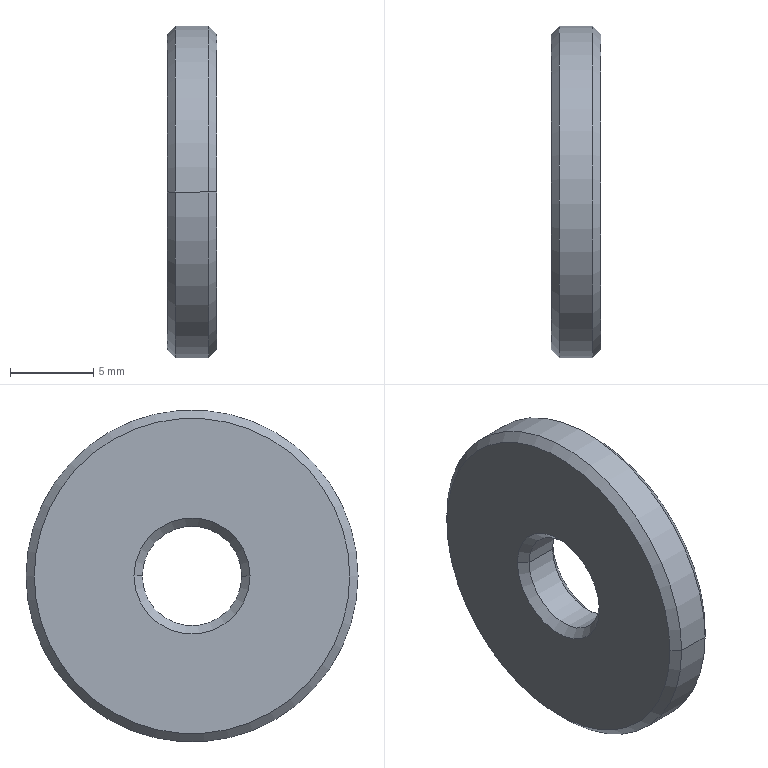Part | STEP file | 0245_005_WSSB20-6-3 | 1 solid | 14 faces | box 3 x 20 x 20 mm | volume 837.234 mm3 | cone 8 | cylinder 4 | plane 2 | commonest cylinder face diameters 6 x2 20 x2
STEP:
#1=CARTESIAN_POINT('',(0.,0.,0.));
#2=DIRECTION('',(0.,0.,1.));
#3=DIRECTION('',(1.,0.,0.));
#4=AXIS2_PLACEMENT_3D('',#1,#2,#3);
#5=CARTESIAN_POINT('',(0.5,-3.,0.));
#6=VERTEX_POINT('',#5);
#7=CARTESIAN_POINT('',(0.,-3.5,0.));
#8=VERTEX_POINT('',#7);
#9=CARTESIAN_POINT('',(0.,-3.5,0.));
#10=DIRECTION('',(-0.7071,-0.7071,0.));
#11=VECTOR('',#10,1.);
#12=LINE('',#9,#11);
#13=CARTESIAN_POINT('',(0.,0.,0.));
#14=DIRECTION('',(-1.,0.,0.));
#15=DIRECTION('',(0.,-1.,0.));
#16=AXIS2_PLACEMENT_3D('',#13,#14,#15);
#17=CONICAL_SURFACE('',#16,3.5,0.7854);
#18=CARTESIAN_POINT('',(6.283,0.));
#19=DIRECTION('',(0.,1.));
#20=VECTOR('',#19,1.);
#21=LINE('',#18,#20);
#22=(GEOMETRIC_REPRESENTATION_CONTEXT(2)PARAMETRIC_REPRESENTATION_CONTEXT()REPRESENTATION_CONTEXT('',''));
#23=DEFINITIONAL_REPRESENTATION('',(#21),#22);
#24=PCURVE('',#17,#23);
#25=CARTESIAN_POINT('',(0.,0.,0.));
#26=DIRECTION('',(-1.,0.,0.));
#27=DIRECTION('',(0.,-1.,0.));
#28=AXIS2_PLACEMENT_3D('',#25,#26,#27);
#29=CONICAL_SURFACE('',#28,3.5,0.7854);
#30=CARTESIAN_POINT('',(0.,0.));
#31=DIRECTION('',(0.,1.));
#32=VECTOR('',#31,1.);
#33=LINE('',#30,#32);
#34=(GEOMETRIC_REPRESENTATION_CONTEXT(2)PARAMETRIC_REPRESENTATION_CONTEXT()REPRESENTATION_CONTEXT('',''));
#35=DEFINITIONAL_REPRESENTATION('',(#33),#34);
#36=PCURVE('',#29,#35);
#37=SURFACE_CURVE('',#12,(#24,#36),.PCURVE_S1.);
#38=EDGE_CURVE('',#6,#8,#37,.T.);
#39=ORIENTED_EDGE('',*,*,#38,.T.);
#40=CARTESIAN_POINT('',(0.,3.5,0.));
#41=VERTEX_POINT('',#40);
#42=CARTESIAN_POINT('',(0.,0.,0.));
#43=DIRECTION('',(1.,0.,0.));
#44=DIRECTION('',(0.,-1.,0.));
#45=AXIS2_PLACEMENT_3D('',#42,#43,#44);
#46=CIRCLE('',#45,3.5);
#47=CARTESIAN_POINT('',(6.283,0.));
#48=DIRECTION('',(-1.,0.));
#49=VECTOR('',#48,1.);
#50=LINE('',#47,#49);
#51=(GEOMETRIC_REPRESENTATION_CONTEXT(2)PARAMETRIC_REPRESENTATION_CONTEXT()REPRESENTATION_CONTEXT('',''));
#52=DEFINITIONAL_REPRESENTATION('',(#50),#51);
#53=PCURVE('',#17,#52);
#54=CARTESIAN_POINT('',(0.,-6.5,0.));
#55=DIRECTION('',(-1.,0.,0.));
#56=DIRECTION('',(0.,-1.,0.));
#57=AXIS2_PLACEMENT_3D('',#54,#55,#56);
#58=PLANE('',#57);
#59=CARTESIAN_POINT('',(-3.,0.));
#60=CARTESIAN_POINT('',(-3.,-6.062));
#61=CARTESIAN_POINT('',(-8.25,-3.031));
#62=CARTESIAN_POINT('',(-13.5,0.));
#63=CARTESIAN_POINT('',(-8.25,3.031));
#64=CARTESIAN_POINT('',(-3.,6.062));
#65=CARTESIAN_POINT('',(-3.,0.));
#66=(BOUNDED_CURVE()B_SPLINE_CURVE(2,(#59,#60,#61,#62,#63,#64,#65),.UNSPECIFIED.,.T.,.F.)B_SPLINE_CURVE_WITH_KNOTS((1,2,2,2,2,1),(-2.094,0.,2.094,4.189,6.283,8.378),.UNSPECIFIED.)CURVE()GEOMETRIC_REPRESENTATION_ITEM()RATIONAL_B_SPLINE_CURVE((1.,0.5,1.,0.5,1.,0.5,1.))REPRESENTATION_ITEM(''));
#67=(GEOMETRIC_REPRESENTATION_CONTEXT(2)PARAMETRIC_REPRESENTATION_CONTEXT()REPRESENTATION_CONTEXT('',''));
#68=DEFINITIONAL_REPRESENTATION('',(#66),#67);
#69=PCURVE('',#58,#68);
#70=SURFACE_CURVE('',#46,(#53,#69),.PCURVE_S1.);
#71=EDGE_CURVE('',#8,#41,#70,.T.);
#72=ORIENTED_EDGE('',*,*,#71,.T.);
#73=CARTESIAN_POINT('',(0.5,3.,0.));
#74=VERTEX_POINT('',#73);
#75=CARTESIAN_POINT('',(0.,3.5,0.));
#76=DIRECTION('',(-0.7071,0.7071,0.));
#77=VECTOR('',#76,1.);
#78=LINE('',#75,#77);
#79=CARTESIAN_POINT('',(3.142,0.));
#80=DIRECTION('',(0.,1.));
#81=VECTOR('',#80,1.);
#82=LINE('',#79,#81);
#83=(GEOMETRIC_REPRESENTATION_CONTEXT(2)PARAMETRIC_REPRESENTATION_CONTEXT()REPRESENTATION_CONTEXT('',''));
#84=DEFINITIONAL_REPRESENTATION('',(#82),#83);
#85=PCURVE('',#17,#84);
#86=CARTESIAN_POINT('',(3.142,0.));
#87=DIRECTION('',(0.,1.));
#88=VECTOR('',#87,1.);
#89=LINE('',#86,#88);
#90=(GEOMETRIC_REPRESENTATION_CONTEXT(2)PARAMETRIC_REPRESENTATION_CONTEXT()REPRESENTATION_CONTEXT('',''));
#91=DEFINITIONAL_REPRESENTATION('',(#89),#90);
#92=PCURVE('',#29,#91);
#93=SURFACE_CURVE('',#78,(#85,#92),.PCURVE_S1.);
#94=EDGE_CURVE('',#74,#41,#93,.T.);
#95=ORIENTED_EDGE('',*,*,#94,.F.);
#96=CARTESIAN_POINT('',(0.5,0.,0.));
#97=DIRECTION('',(-1.,0.,0.));
#98=DIRECTION('',(0.,-1.,0.));
#99=AXIS2_PLACEMENT_3D('',#96,#97,#98);
#100=CIRCLE('',#99,3.);
#101=CARTESIAN_POINT('',(0.,-0.5));
#102=DIRECTION('',(1.,0.));
#103=VECTOR('',#102,1.);
#104=LINE('',#101,#103);
#105=(GEOMETRIC_REPRESENTATION_CONTEXT(2)PARAMETRIC_REPRESENTATION_CONTEXT()REPRESENTATION_CONTEXT('',''));
#106=DEFINITIONAL_REPRESENTATION('',(#104),#105);
#107=PCURVE('',#17,#106);
#108=CARTESIAN_POINT('',(1.5,0.,0.));
#109=DIRECTION('',(-1.,0.,0.));
#110=DIRECTION('',(0.,-1.,0.));
#111=AXIS2_PLACEMENT_3D('',#108,#109,#110);
#112=CYLINDRICAL_SURFACE('',#111,3.);
#113=CARTESIAN_POINT('',(0.,1.));
#114=DIRECTION('',(1.,0.));
#115=VECTOR('',#114,1.);
#116=LINE('',#113,#115);
#117=(GEOMETRIC_REPRESENTATION_CONTEXT(2)PARAMETRIC_REPRESENTATION_CONTEXT()REPRESENTATION_CONTEXT('',''));
#118=DEFINITIONAL_REPRESENTATION('',(#116),#117);
#119=PCURVE('',#112,#118);
#120=SURFACE_CURVE('',#100,(#107,#119),.PCURVE_S1.);
#121=EDGE_CURVE('',#74,#6,#120,.T.);
#122=ORIENTED_EDGE('',*,*,#121,.T.);
#123=EDGE_LOOP('',(#39,#72,#95,#122));
#124=FACE_BOUND('',#123,.F.);
#125=ADVANCED_FACE('',(#124),#17,.F.);
#126=CARTESIAN_POINT('',(0.,-9.5,0.));
#127=VERTEX_POINT('',#126);
#128=CARTESIAN_POINT('',(0.,9.5,0.));
#129=VERTEX_POINT('',#128);
#130=CARTESIAN_POINT('',(0.,0.,0.));
#131=DIRECTION('',(-1.,0.,0.));
#132=DIRECTION('',(0.,1.,0.));
#133=AXIS2_PLACEMENT_3D('',#130,#131,#132);
#134=CIRCLE('',#133,9.5);
#135=CARTESIAN_POINT('',(0.5,0.,0.));
#136=DIRECTION('',(1.,0.,0.));
#137=DIRECTION('',(0.,1.,0.));
#138=AXIS2_PLACEMENT_3D('',#135,#136,#137);
#139=CONICAL_SURFACE('',#138,10.,0.7854);
#140=CARTESIAN_POINT('',(6.283,-0.5));
#141=DIRECTION('',(-1.,0.));
#142=VECTOR('',#141,1.);
#143=LINE('',#140,#142);
#144=(GEOMETRIC_REPRESENTATION_CONTEXT(2)PARAMETRIC_REPRESENTATION_CONTEXT()REPRESENTATION_CONTEXT('',''));
#145=DEFINITIONAL_REPRESENTATION('',(#143),#144);
#146=PCURVE('',#139,#145);
#147=CARTESIAN_POINT('',(-6.5,0.));
#148=DIRECTION('',(-1.,0.));
#149=AXIS2_PLACEMENT_2D('',#147,#148);
#150=CIRCLE('',#149,9.5);
#151=(GEOMETRIC_REPRESENTATION_CONTEXT(2)PARAMETRIC_REPRESENTATION_CONTEXT()REPRESENTATION_CONTEXT('',''));
#152=DEFINITIONAL_REPRESENTATION('',(#150),#151);
#153=PCURVE('',#58,#152);
#154=SURFACE_CURVE('',#134,(#146,#153),.PCURVE_S1.);
#155=EDGE_CURVE('',#127,#129,#154,.T.);
#156=ORIENTED_EDGE('',*,*,#155,.F.);
#157=CARTESIAN_POINT('',(0.5,-10.,0.));
#158=VERTEX_POINT('',#157);
#159=CARTESIAN_POINT('',(0.5,-10.,0.));
#160=DIRECTION('',(0.7071,-0.7071,0.));
#161=VECTOR('',#160,1.);
#162=LINE('',#159,#161);
#163=CARTESIAN_POINT('',(3.142,0.));
#164=DIRECTION('',(0.,1.));
#165=VECTOR('',#164,1.);
#166=LINE('',#163,#165);
#167=(GEOMETRIC_REPRESENTATION_CONTEXT(2)PARAMETRIC_REPRESENTATION_CONTEXT()REPRESENTATION_CONTEXT('',''));
#168=DEFINITIONAL_REPRESENTATION('',(#166),#167);
#169=PCURVE('',#139,#168);
#170=CARTESIAN_POINT('',(0.5,0.,0.));
#171=DIRECTION('',(1.,0.,0.));
#172=DIRECTION('',(0.,1.,0.));
#173=AXIS2_PLACEMENT_3D('',#170,#171,#172);
#174=CONICAL_SURFACE('',#173,10.,0.7854);
#175=CARTESIAN_POINT('',(3.142,0.));
#176=DIRECTION('',(0.,1.));
#177=VECTOR('',#176,1.);
#178=LINE('',#175,#177);
#179=(GEOMETRIC_REPRESENTATION_CONTEXT(2)PARAMETRIC_REPRESENTATION_CONTEXT()REPRESENTATION_CONTEXT('',''));
#180=DEFINITIONAL_REPRESENTATION('',(#178),#179);
#181=PCURVE('',#174,#180);
#182=SURFACE_CURVE('',#162,(#169,#181),.PCURVE_S1.);
#183=EDGE_CURVE('',#127,#158,#182,.T.);
#184=ORIENTED_EDGE('',*,*,#183,.T.);
#185=CARTESIAN_POINT('',(0.5,10.,0.));
#186=VERTEX_POINT('',#185);
#187=CARTESIAN_POINT('',(0.5,0.,0.));
#188=DIRECTION('',(-1.,0.,0.));
#189=DIRECTION('',(0.,-1.,0.));
#190=AXIS2_PLACEMENT_3D('',#187,#188,#189);
#191=CIRCLE('',#190,10.);
#192=CARTESIAN_POINT('',(3.142,0.));
#193=DIRECTION('',(-1.,0.));
#194=VECTOR('',#193,1.);
#195=LINE('',#192,#194);
#196=(GEOMETRIC_REPRESENTATION_CONTEXT(2)PARAMETRIC_REPRESENTATION_CONTEXT()REPRESENTATION_CONTEXT('',''));
#197=DEFINITIONAL_REPRESENTATION('',(#195),#196);
#198=PCURVE('',#139,#197);
#199=CARTESIAN_POINT('',(1.5,0.,0.));
#200=DIRECTION('',(-1.,0.,0.));
#201=DIRECTION('',(0.,-1.,0.));
#202=AXIS2_PLACEMENT_3D('',#199,#200,#201);
#203=CYLINDRICAL_SURFACE('',#202,10.);
#204=CARTESIAN_POINT('',(0.,1.));
#205=DIRECTION('',(1.,0.));
#206=VECTOR('',#205,1.);
#207=LINE('',#204,#206);
#208=(GEOMETRIC_REPRESENTATION_CONTEXT(2)PARAMETRIC_REPRESENTATION_CONTEXT()REPRESENTATION_CONTEXT('',''));
#209=DEFINITIONAL_REPRESENTATION('',(#207),#208);
#210=PCURVE('',#203,#209);
#211=SURFACE_CURVE('',#191,(#198,#210),.PCURVE_S1.);
#212=EDGE_CURVE('',#158,#186,#211,.T.);
#213=ORIENTED_EDGE('',*,*,#212,.T.);
#214=CARTESIAN_POINT('',(0.5,10.,0.));
#215=DIRECTION('',(0.7071,0.7071,0.));
#216=VECTOR('',#215,1.);
#217=LINE('',#214,#216);
#218=CARTESIAN_POINT('',(0.,0.));
#219=DIRECTION('',(0.,1.));
#220=VECTOR('',#219,1.);
#221=LINE('',#218,#220);
#222=(GEOMETRIC_REPRESENTATION_CONTEXT(2)PARAMETRIC_REPRESENTATION_CONTEXT()REPRESENTATION_CONTEXT('',''));
#223=DEFINITIONAL_REPRESENTATION('',(#221),#222);
#224=PCURVE('',#139,#223);
#225=CARTESIAN_POINT('',(6.283,0.));
#226=DIRECTION('',(0.,1.));
#227=VECTOR('',#226,1.);
#228=LINE('',#225,#227);
#229=(GEOMETRIC_REPRESENTATION_CONTEXT(2)PARAMETRIC_REPRESENTATION_CONTEXT()REPRESENTATION_CONTEXT('',''));
#230=DEFINITIONAL_REPRESENTATION('',(#228),#229);
#231=PCURVE('',#174,#230);
#232=SURFACE_CURVE('',#217,(#224,#231),.PCURVE_S1.);
#233=EDGE_CURVE('',#129,#186,#232,.T.);
#234=ORIENTED_EDGE('',*,*,#233,.F.);
#235=EDGE_LOOP('',(#156,#184,#213,#234));
#236=FACE_BOUND('',#235,.T.);
#237=ADVANCED_FACE('',(#236),#139,.T.);
#238=CARTESIAN_POINT('',(2.5,-3.,0.));
#239=VERTEX_POINT('',#238);
#240=CARTESIAN_POINT('',(1.5,-3.,0.));
#241=DIRECTION('',(-1.,0.,0.));
#242=VECTOR('',#241,1.);
#243=LINE('',#240,#242);
#244=CARTESIAN_POINT('',(6.283,0.));
#245=DIRECTION('',(0.,1.));
#246=VECTOR('',#245,1.);
#247=LINE('',#244,#246);
#248=(GEOMETRIC_REPRESENTATION_CONTEXT(2)PARAMETRIC_REPRESENTATION_CONTEXT()REPRESENTATION_CONTEXT('',''));
#249=DEFINITIONAL_REPRESENTATION('',(#247),#248);
#250=PCURVE('',#112,#249);
#251=CARTESIAN_POINT('',(1.5,0.,0.));
#252=DIRECTION('',(-1.,0.,0.));
#253=DIRECTION('',(0.,-1.,0.));
#254=AXIS2_PLACEMENT_3D('',#251,#252,#253);
#255=CYLINDRICAL_SURFACE('',#254,3.);
#256=CARTESIAN_POINT('',(0.,0.));
#257=DIRECTION('',(0.,1.));
#258=VECTOR('',#257,1.);
#259=LINE('',#256,#258);
#260=(GEOMETRIC_REPRESENTATION_CONTEXT(2)PARAMETRIC_REPRESENTATION_CONTEXT()REPRESENTATION_CONTEXT('',''));
#261=DEFINITIONAL_REPRESENTATION('',(#259),#260);
#262=PCURVE('',#255,#261);
#263=SURFACE_CURVE('',#243,(#250,#262),.PCURVE_S1.);
#264=EDGE_CURVE('',#239,#6,#263,.T.);
#265=ORIENTED_EDGE('',*,*,#264,.T.);
#266=ORIENTED_EDGE('',*,*,#121,.F.);
#267=CARTESIAN_POINT('',(2.5,3.,0.));
#268=VERTEX_POINT('',#267);
#269=CARTESIAN_POINT('',(1.5,3.,0.));
#270=DIRECTION('',(-1.,0.,0.));
#271=VECTOR('',#270,1.);
#272=LINE('',#269,#271);
#273=CARTESIAN_POINT('',(3.142,0.));
#274=DIRECTION('',(0.,1.));
#275=VECTOR('',#274,1.);
#276=LINE('',#273,#275);
#277=(GEOMETRIC_REPRESENTATION_CONTEXT(2)PARAMETRIC_REPRESENTATION_CONTEXT()REPRESENTATION_CONTEXT('',''));
#278=DEFINITIONAL_REPRESENTATION('',(#276),#277);
#279=PCURVE('',#112,#278);
#280=CARTESIAN_POINT('',(3.142,0.));
#281=DIRECTION('',(0.,1.));
#282=VECTOR('',#281,1.);
#283=LINE('',#280,#282);
#284=(GEOMETRIC_REPRESENTATION_CONTEXT(2)PARAMETRIC_REPRESENTATION_CONTEXT()REPRESENTATION_CONTEXT('',''));
#285=DEFINITIONAL_REPRESENTATION('',(#283),#284);
#286=PCURVE('',#255,#285);
#287=SURFACE_CURVE('',#272,(#279,#286),.PCURVE_S1.);
#288=EDGE_CURVE('',#268,#74,#287,.T.);
#289=ORIENTED_EDGE('',*,*,#288,.F.);
#290=CARTESIAN_POINT('',(2.5,0.,0.));
#291=DIRECTION('',(-1.,0.,0.));
#292=DIRECTION('',(0.,-1.,0.));
#293=AXIS2_PLACEMENT_3D('',#290,#291,#292);
#294=CIRCLE('',#293,3.);
#295=CARTESIAN_POINT('',(0.,-1.));
#296=DIRECTION('',(1.,0.));
#297=VECTOR('',#296,1.);
#298=LINE('',#295,#297);
#299=(GEOMETRIC_REPRESENTATION_CONTEXT(2)PARAMETRIC_REPRESENTATION_CONTEXT()REPRESENTATION_CONTEXT('',''));
#300=DEFINITIONAL_REPRESENTATION('',(#298),#299);
#301=PCURVE('',#112,#300);
#302=CARTESIAN_POINT('',(3.,0.,0.));
#303=DIRECTION('',(1.,0.,0.));
#304=DIRECTION('',(0.,1.,0.));
#305=AXIS2_PLACEMENT_3D('',#302,#303,#304);
#306=CONICAL_SURFACE('',#305,3.5,0.7854);
#307=CARTESIAN_POINT('',(9.425,-0.5));
#308=DIRECTION('',(-1.,0.));
#309=VECTOR('',#308,1.);
#310=LINE('',#307,#309);
#311=(GEOMETRIC_REPRESENTATION_CONTEXT(2)PARAMETRIC_REPRESENTATION_CONTEXT()REPRESENTATION_CONTEXT('',''));
#312=DEFINITIONAL_REPRESENTATION('',(#310),#311);
#313=PCURVE('',#306,#312);
#314=SURFACE_CURVE('',#294,(#301,#313),.PCURVE_S1.);
#315=EDGE_CURVE('',#268,#239,#314,.T.);
#316=ORIENTED_EDGE('',*,*,#315,.T.);
#317=EDGE_LOOP('',(#265,#266,#289,#316));
#318=FACE_BOUND('',#317,.F.);
#319=ADVANCED_FACE('',(#318),#112,.F.);
#320=CARTESIAN_POINT('',(2.5,-10.,0.));
#321=VERTEX_POINT('',#320);
#322=CARTESIAN_POINT('',(2.5,10.,0.));
#323=VERTEX_POINT('',#322);
#324=CARTESIAN_POINT('',(2.5,0.,0.));
#325=DIRECTION('',(-1.,0.,0.));
#326=DIRECTION('',(0.,-1.,0.));
#327=AXIS2_PLACEMENT_3D('',#324,#325,#326);
#328=CIRCLE('',#327,10.);
#329=CARTESIAN_POINT('',(0.,-1.));
#330=DIRECTION('',(1.,0.));
#331=VECTOR('',#330,1.);
#332=LINE('',#329,#331);
#333=(GEOMETRIC_REPRESENTATION_CONTEXT(2)PARAMETRIC_REPRESENTATION_CONTEXT()REPRESENTATION_CONTEXT('',''));
#334=DEFINITIONAL_REPRESENTATION('',(#332),#333);
#335=PCURVE('',#203,#334);
#336=CARTESIAN_POINT('',(2.5,0.,0.));
#337=DIRECTION('',(-1.,0.,0.));
#338=DIRECTION('',(0.,-1.,0.));
#339=AXIS2_PLACEMENT_3D('',#336,#337,#338);
#340=CONICAL_SURFACE('',#339,10.,0.7854);
#341=CARTESIAN_POINT('',(0.,0.));
#342=DIRECTION('',(1.,0.));
#343=VECTOR('',#342,1.);
#344=LINE('',#341,#343);
#345=(GEOMETRIC_REPRESENTATION_CONTEXT(2)PARAMETRIC_REPRESENTATION_CONTEXT()REPRESENTATION_CONTEXT('',''));
#346=DEFINITIONAL_REPRESENTATION('',(#344),#345);
#347=PCURVE('',#340,#346);
#348=SURFACE_CURVE('',#328,(#335,#347),.PCURVE_S1.);
#349=EDGE_CURVE('',#321,#323,#348,.T.);
#350=ORIENTED_EDGE('',*,*,#349,.T.);
#351=CARTESIAN_POINT('',(1.5,10.,0.));
#352=DIRECTION('',(-1.,0.,0.));
#353=VECTOR('',#352,1.);
#354=LINE('',#351,#353);
#355=CARTESIAN_POINT('',(3.142,0.));
#356=DIRECTION('',(0.,1.));
#357=VECTOR('',#356,1.);
#358=LINE('',#355,#357);
#359=(GEOMETRIC_REPRESENTATION_CONTEXT(2)PARAMETRIC_REPRESENTATION_CONTEXT()REPRESENTATION_CONTEXT('',''));
#360=DEFINITIONAL_REPRESENTATION('',(#358),#359);
#361=PCURVE('',#203,#360);
#362=CARTESIAN_POINT('',(1.5,0.,0.));
#363=DIRECTION('',(-1.,0.,0.));
#364=DIRECTION('',(0.,-1.,0.));
#365=AXIS2_PLACEMENT_3D('',#362,#363,#364);
#366=CYLINDRICAL_SURFACE('',#365,10.);
#367=CARTESIAN_POINT('',(3.142,0.));
#368=DIRECTION('',(0.,1.));
#369=VECTOR('',#368,1.);
#370=LINE('',#367,#369);
#371=(GEOMETRIC_REPRESENTATION_CONTEXT(2)PARAMETRIC_REPRESENTATION_CONTEXT()REPRESENTATION_CONTEXT('',''));
#372=DEFINITIONAL_REPRESENTATION('',(#370),#371);
#373=PCURVE('',#366,#372);
#374=SURFACE_CURVE('',#354,(#361,#373),.PCURVE_S1.);
#375=EDGE_CURVE('',#323,#186,#374,.T.);
#376=ORIENTED_EDGE('',*,*,#375,.T.);
#377=ORIENTED_EDGE('',*,*,#212,.F.);
#378=CARTESIAN_POINT('',(1.5,-10.,0.));
#379=DIRECTION('',(-1.,0.,0.));
#380=VECTOR('',#379,1.);
#381=LINE('',#378,#380);
#382=CARTESIAN_POINT('',(0.,0.));
#383=DIRECTION('',(0.,1.));
#384=VECTOR('',#383,1.);
#385=LINE('',#382,#384);
#386=(GEOMETRIC_REPRESENTATION_CONTEXT(2)PARAMETRIC_REPRESENTATION_CONTEXT()REPRESENTATION_CONTEXT('',''));
#387=DEFINITIONAL_REPRESENTATION('',(#385),#386);
#388=PCURVE('',#203,#387);
#389=CARTESIAN_POINT('',(6.283,0.));
#390=DIRECTION('',(0.,1.));
#391=VECTOR('',#390,1.);
#392=LINE('',#389,#391);
#393=(GEOMETRIC_REPRESENTATION_CONTEXT(2)PARAMETRIC_REPRESENTATION_CONTEXT()REPRESENTATION_CONTEXT('',''));
#394=DEFINITIONAL_REPRESENTATION('',(#392),#393);
#395=PCURVE('',#366,#394);
#396=SURFACE_CURVE('',#381,(#388,#395),.PCURVE_S1.);
#397=EDGE_CURVE('',#321,#158,#396,.T.);
#398=ORIENTED_EDGE('',*,*,#397,.F.);
#399=EDGE_LOOP('',(#350,#376,#377,#398));
#400=FACE_BOUND('',#399,.T.);
#401=ADVANCED_FACE('',(#400),#203,.T.);
#402=CARTESIAN_POINT('',(3.,3.5,0.));
#403=VERTEX_POINT('',#402);
#404=CARTESIAN_POINT('',(3.,3.5,0.));
#405=DIRECTION('',(0.7071,0.7071,0.));
#406=VECTOR('',#405,1.);
#407=LINE('',#404,#406);
#408=CARTESIAN_POINT('',(6.283,0.));
#409=DIRECTION('',(0.,1.));
#410=VECTOR('',#409,1.);
#411=LINE('',#408,#410);
#412=(GEOMETRIC_REPRESENTATION_CONTEXT(2)PARAMETRIC_REPRESENTATION_CONTEXT()REPRESENTATION_CONTEXT('',''));
#413=DEFINITIONAL_REPRESENTATION('',(#411),#412);
#414=PCURVE('',#306,#413);
#415=CARTESIAN_POINT('',(3.,0.,0.));
#416=DIRECTION('',(1.,0.,0.));
#417=DIRECTION('',(0.,1.,0.));
#418=AXIS2_PLACEMENT_3D('',#415,#416,#417);
#419=CONICAL_SURFACE('',#418,3.5,0.7854);
#420=CARTESIAN_POINT('',(0.,0.));
#421=DIRECTION('',(0.,1.));
#422=VECTOR('',#421,1.);
#423=LINE('',#420,#422);
#424=(GEOMETRIC_REPRESENTATION_CONTEXT(2)PARAMETRIC_REPRESENTATION_CONTEXT()REPRESENTATION_CONTEXT('',''));
#425=DEFINITIONAL_REPRESENTATION('',(#423),#424);
#426=PCURVE('',#419,#425);
#427=SURFACE_CURVE('',#407,(#414,#426),.PCURVE_S1.);
#428=EDGE_CURVE('',#268,#403,#427,.T.);
#429=ORIENTED_EDGE('',*,*,#428,.T.);
#430=CARTESIAN_POINT('',(3.,-3.5,0.));
#431=VERTEX_POINT('',#430);
#432=CARTESIAN_POINT('',(3.,0.,0.));
#433=DIRECTION('',(-1.,0.,0.));
#434=DIRECTION('',(0.,1.,0.));
#435=AXIS2_PLACEMENT_3D('',#432,#433,#434);
#436=CIRCLE('',#435,3.5);
#437=CARTESIAN_POINT('',(6.283,0.));
#438=DIRECTION('',(-1.,0.));
#439=VECTOR('',#438,1.);
#440=LINE('',#437,#439);
#441=(GEOMETRIC_REPRESENTATION_CONTEXT(2)PARAMETRIC_REPRESENTATION_CONTEXT()REPRESENTATION_CONTEXT('',''));
#442=DEFINITIONAL_REPRESENTATION('',(#440),#441);
#443=PCURVE('',#306,#442);
#444=CARTESIAN_POINT('',(3.,-6.5,0.));
#445=DIRECTION('',(1.,0.,0.));
#446=DIRECTION('',(0.,1.,0.));
#447=AXIS2_PLACEMENT_3D('',#444,#445,#446);
#448=PLANE('',#447);
#449=CARTESIAN_POINT('',(10.,0.));
#450=CARTESIAN_POINT('',(10.,-6.062));
#451=CARTESIAN_POINT('',(4.75,-3.031));
#452=CARTESIAN_POINT('',(-0.5,0.));
#453=CARTESIAN_POINT('',(4.75,3.031));
#454=CARTESIAN_POINT('',(10.,6.062));
#455=CARTESIAN_POINT('',(10.,0.));
#456=(BOUNDED_CURVE()B_SPLINE_CURVE(2,(#449,#450,#451,#452,#453,#454,#455),.UNSPECIFIED.,.T.,.F.)B_SPLINE_CURVE_WITH_KNOTS((1,2,2,2,2,1),(-2.094,0.,2.094,4.189,6.283,8.378),.UNSPECIFIED.)CURVE()GEOMETRIC_REPRESENTATION_ITEM()RATIONAL_B_SPLINE_CURVE((1.,0.5,1.,0.5,1.,0.5,1.))REPRESENTATION_ITEM(''));
#457=(GEOMETRIC_REPRESENTATION_CONTEXT(2)PARAMETRIC_REPRESENTATION_CONTEXT()REPRESENTATION_CONTEXT('',''));
#458=DEFINITIONAL_REPRESENTATION('',(#456),#457);
#459=PCURVE('',#448,#458);
#460=SURFACE_CURVE('',#436,(#443,#459),.PCURVE_S1.);
#461=EDGE_CURVE('',#403,#431,#460,.T.);
#462=ORIENTED_EDGE('',*,*,#461,.T.);
#463=CARTESIAN_POINT('',(3.,-3.5,0.));
#464=DIRECTION('',(0.7071,-0.7071,0.));
#465=VECTOR('',#464,1.);
#466=LINE('',#463,#465);
#467=CARTESIAN_POINT('',(3.142,0.));
#468=DIRECTION('',(0.,1.));
#469=VECTOR('',#468,1.);
#470=LINE('',#467,#469);
#471=(GEOMETRIC_REPRESENTATION_CONTEXT(2)PARAMETRIC_REPRESENTATION_CONTEXT()REPRESENTATION_CONTEXT('',''));
#472=DEFINITIONAL_REPRESENTATION('',(#470),#471);
#473=PCURVE('',#306,#472);
#474=CARTESIAN_POINT('',(3.142,0.));
#475=DIRECTION('',(0.,1.));
#476=VECTOR('',#475,1.);
#477=LINE('',#474,#476);
#478=(GEOMETRIC_REPRESENTATION_CONTEXT(2)PARAMETRIC_REPRESENTATION_CONTEXT()REPRESENTATION_CONTEXT('',''));
#479=DEFINITIONAL_REPRESENTATION('',(#477),#478);
#480=PCURVE('',#419,#479);
#481=SURFACE_CURVE('',#466,(#473,#480),.PCURVE_S1.);
#482=EDGE_CURVE('',#239,#431,#481,.T.);
#483=ORIENTED_EDGE('',*,*,#482,.F.);
#484=ORIENTED_EDGE('',*,*,#315,.F.);
#485=EDGE_LOOP('',(#429,#462,#483,#484));
#486=FACE_BOUND('',#485,.F.);
#487=ADVANCED_FACE('',(#486),#306,.F.);
#488=CARTESIAN_POINT('',(3.,-9.5,0.));
#489=VERTEX_POINT('',#488);
#490=CARTESIAN_POINT('',(3.,9.5,0.));
#491=VERTEX_POINT('',#490);
#492=CARTESIAN_POINT('',(3.,0.,0.));
#493=DIRECTION('',(-1.,0.,0.));
#494=DIRECTION('',(0.,-1.,0.));
#495=AXIS2_PLACEMENT_3D('',#492,#493,#494);
#496=CIRCLE('',#495,9.5);
#497=CARTESIAN_POINT('',(0.,-0.5));
#498=DIRECTION('',(1.,0.));
#499=VECTOR('',#498,1.);
#500=LINE('',#497,#499);
#501=(GEOMETRIC_REPRESENTATION_CONTEXT(2)PARAMETRIC_REPRESENTATION_CONTEXT()REPRESENTATION_CONTEXT('',''));
#502=DEFINITIONAL_REPRESENTATION('',(#500),#501);
#503=PCURVE('',#340,#502);
#504=CARTESIAN_POINT('',(-3.,0.));
#505=CARTESIAN_POINT('',(-3.,16.454));
#506=CARTESIAN_POINT('',(11.25,8.227));
#507=CARTESIAN_POINT('',(25.5,0.));
#508=CARTESIAN_POINT('',(11.25,-8.227));
#509=CARTESIAN_POINT('',(-3.,-16.454));
#510=CARTESIAN_POINT('',(-3.,0.));
#511=(BOUNDED_CURVE()B_SPLINE_CURVE(2,(#504,#505,#506,#507,#508,#509,#510),.UNSPECIFIED.,.T.,.F.)B_SPLINE_CURVE_WITH_KNOTS((1,2,2,2,2,1),(-2.094,0.,2.094,4.189,6.283,8.378),.UNSPECIFIED.)CURVE()GEOMETRIC_REPRESENTATION_ITEM()RATIONAL_B_SPLINE_CURVE((1.,0.5,1.,0.5,1.,0.5,1.))REPRESENTATION_ITEM(''));
#512=(GEOMETRIC_REPRESENTATION_CONTEXT(2)PARAMETRIC_REPRESENTATION_CONTEXT()REPRESENTATION_CONTEXT('',''));
#513=DEFINITIONAL_REPRESENTATION('',(#511),#512);
#514=PCURVE('',#448,#513);
#515=SURFACE_CURVE('',#496,(#503,#514),.PCURVE_S1.);
#516=EDGE_CURVE('',#489,#491,#515,.T.);
#517=ORIENTED_EDGE('',*,*,#516,.T.);
#518=CARTESIAN_POINT('',(2.5,10.,0.));
#519=DIRECTION('',(-0.7071,0.7071,0.));
#520=VECTOR('',#519,1.);
#521=LINE('',#518,#520);
#522=CARTESIAN_POINT('',(3.142,0.));
#523=DIRECTION('',(0.,1.));
#524=VECTOR('',#523,1.);
#525=LINE('',#522,#524);
#526=(GEOMETRIC_REPRESENTATION_CONTEXT(2)PARAMETRIC_REPRESENTATION_CONTEXT()REPRESENTATION_CONTEXT('',''));
#527=DEFINITIONAL_REPRESENTATION('',(#525),#526);
#528=PCURVE('',#340,#527);
#529=CARTESIAN_POINT('',(2.5,0.,0.));
#530=DIRECTION('',(-1.,0.,0.));
#531=DIRECTION('',(0.,-1.,0.));
#532=AXIS2_PLACEMENT_3D('',#529,#530,#531);
#533=CONICAL_SURFACE('',#532,10.,0.7854);
#534=CARTESIAN_POINT('',(3.142,0.));
#535=DIRECTION('',(0.,1.));
#536=VECTOR('',#535,1.);
#537=LINE('',#534,#536);
#538=(GEOMETRIC_REPRESENTATION_CONTEXT(2)PARAMETRIC_REPRESENTATION_CONTEXT()REPRESENTATION_CONTEXT('',''));
#539=DEFINITIONAL_REPRESENTATION('',(#537),#538);
#540=PCURVE('',#533,#539);
#541=SURFACE_CURVE('',#521,(#528,#540),.PCURVE_S1.);
#542=EDGE_CURVE('',#491,#323,#541,.T.);
#543=ORIENTED_EDGE('',*,*,#542,.T.);
#544=ORIENTED_EDGE('',*,*,#349,.F.);
#545=CARTESIAN_POINT('',(2.5,-10.,0.));
#546=DIRECTION('',(-0.7071,-0.7071,0.));
#547=VECTOR('',#546,1.);
#548=LINE('',#545,#547);
#549=CARTESIAN_POINT('',(0.,0.));
#550=DIRECTION('',(0.,1.));
#551=VECTOR('',#550,1.);
#552=LINE('',#549,#551);
#553=(GEOMETRIC_REPRESENTATION_CONTEXT(2)PARAMETRIC_REPRESENTATION_CONTEXT()REPRESENTATION_CONTEXT('',''));
#554=DEFINITIONAL_REPRESENTATION('',(#552),#553);
#555=PCURVE('',#340,#554);
#556=CARTESIAN_POINT('',(6.283,0.));
#557=DIRECTION('',(0.,1.));
#558=VECTOR('',#557,1.);
#559=LINE('',#556,#558);
#560=(GEOMETRIC_REPRESENTATION_CONTEXT(2)PARAMETRIC_REPRESENTATION_CONTEXT()REPRESENTATION_CONTEXT('',''));
#561=DEFINITIONAL_REPRESENTATION('',(#559),#560);
#562=PCURVE('',#533,#561);
#563=SURFACE_CURVE('',#548,(#555,#562),.PCURVE_S1.);
#564=EDGE_CURVE('',#489,#321,#563,.T.);
#565=ORIENTED_EDGE('',*,*,#564,.F.);
#566=EDGE_LOOP('',(#517,#543,#544,#565));
#567=FACE_BOUND('',#566,.T.);
#568=ADVANCED_FACE('',(#567),#340,.T.);
#569=ORIENTED_EDGE('',*,*,#71,.T.);
#570=CARTESIAN_POINT('',(0.,0.,0.));
#571=DIRECTION('',(1.,0.,0.));
#572=DIRECTION('',(0.,-1.,0.));
#573=AXIS2_PLACEMENT_3D('',#570,#571,#572);
#574=CIRCLE('',#573,3.5);
#575=CARTESIAN_POINT('',(-3.,0.));
#576=CARTESIAN_POINT('',(-3.,-6.062));
#577=CARTESIAN_POINT('',(-8.25,-3.031));
#578=CARTESIAN_POINT('',(-13.5,0.));
#579=CARTESIAN_POINT('',(-8.25,3.031));
#580=CARTESIAN_POINT('',(-3.,6.062));
#581=CARTESIAN_POINT('',(-3.,0.));
#582=(BOUNDED_CURVE()B_SPLINE_CURVE(2,(#575,#576,#577,#578,#579,#580,#581),.UNSPECIFIED.,.T.,.F.)B_SPLINE_CURVE_WITH_KNOTS((1,2,2,2,2,1),(-2.094,0.,2.094,4.189,6.283,8.378),.UNSPECIFIED.)CURVE()GEOMETRIC_REPRESENTATION_ITEM()RATIONAL_B_SPLINE_CURVE((1.,0.5,1.,0.5,1.,0.5,1.))REPRESENTATION_ITEM(''));
#583=(GEOMETRIC_REPRESENTATION_CONTEXT(2)PARAMETRIC_REPRESENTATION_CONTEXT()REPRESENTATION_CONTEXT('',''));
#584=DEFINITIONAL_REPRESENTATION('',(#582),#583);
#585=PCURVE('',#58,#584);
#586=CARTESIAN_POINT('',(6.283,0.));
#587=DIRECTION('',(-1.,0.));
#588=VECTOR('',#587,1.);
#589=LINE('',#586,#588);
#590=(GEOMETRIC_REPRESENTATION_CONTEXT(2)PARAMETRIC_REPRESENTATION_CONTEXT()REPRESENTATION_CONTEXT('',''));
#591=DEFINITIONAL_REPRESENTATION('',(#589),#590);
#592=PCURVE('',#29,#591);
#593=SURFACE_CURVE('',#574,(#585,#592),.PCURVE_S1.);
#594=EDGE_CURVE('',#41,#8,#593,.T.);
#595=ORIENTED_EDGE('',*,*,#594,.T.);
#596=EDGE_LOOP('',(#569,#595));
#597=FACE_BOUND('',#596,.T.);
#598=CARTESIAN_POINT('',(0.,0.,0.));
#599=DIRECTION('',(-1.,0.,0.));
#600=DIRECTION('',(0.,1.,0.));
#601=AXIS2_PLACEMENT_3D('',#598,#599,#600);
#602=CIRCLE('',#601,9.5);
#603=CARTESIAN_POINT('',(-6.5,0.));
#604=DIRECTION('',(-1.,0.));
#605=AXIS2_PLACEMENT_2D('',#603,#604);
#606=CIRCLE('',#605,9.5);
#607=(GEOMETRIC_REPRESENTATION_CONTEXT(2)PARAMETRIC_REPRESENTATION_CONTEXT()REPRESENTATION_CONTEXT('',''));
#608=DEFINITIONAL_REPRESENTATION('',(#606),#607);
#609=PCURVE('',#58,#608);
#610=CARTESIAN_POINT('',(6.283,-0.5));
#611=DIRECTION('',(-1.,0.));
#612=VECTOR('',#611,1.);
#613=LINE('',#610,#612);
#614=(GEOMETRIC_REPRESENTATION_CONTEXT(2)PARAMETRIC_REPRESENTATION_CONTEXT()REPRESENTATION_CONTEXT('',''));
#615=DEFINITIONAL_REPRESENTATION('',(#613),#614);
#616=PCURVE('',#174,#615);
#617=SURFACE_CURVE('',#602,(#609,#616),.PCURVE_S1.);
#618=EDGE_CURVE('',#129,#127,#617,.T.);
#619=ORIENTED_EDGE('',*,*,#618,.T.);
#620=ORIENTED_EDGE('',*,*,#155,.T.);
#621=EDGE_LOOP('',(#619,#620));
#622=FACE_BOUND('',#621,.T.);
#623=ADVANCED_FACE('',(#597,#622),#58,.T.);
#624=ORIENTED_EDGE('',*,*,#594,.T.);
#625=ORIENTED_EDGE('',*,*,#38,.F.);
#626=CARTESIAN_POINT('',(0.5,0.,0.));
#627=DIRECTION('',(-1.,0.,0.));
#628=DIRECTION('',(0.,-1.,0.));
#629=AXIS2_PLACEMENT_3D('',#626,#627,#628);
#630=CIRCLE('',#629,3.);
#631=CARTESIAN_POINT('',(0.,-0.5));
#632=DIRECTION('',(1.,0.));
#633=VECTOR('',#632,1.);
#634=LINE('',#631,#633);
#635=(GEOMETRIC_REPRESENTATION_CONTEXT(2)PARAMETRIC_REPRESENTATION_CONTEXT()REPRESENTATION_CONTEXT('',''));
#636=DEFINITIONAL_REPRESENTATION('',(#634),#635);
#637=PCURVE('',#29,#636);
#638=CARTESIAN_POINT('',(0.,1.));
#639=DIRECTION('',(1.,0.));
#640=VECTOR('',#639,1.);
#641=LINE('',#638,#640);
#642=(GEOMETRIC_REPRESENTATION_CONTEXT(2)PARAMETRIC_REPRESENTATION_CONTEXT()REPRESENTATION_CONTEXT('',''));
#643=DEFINITIONAL_REPRESENTATION('',(#641),#642);
#644=PCURVE('',#255,#643);
#645=SURFACE_CURVE('',#630,(#637,#644),.PCURVE_S1.);
#646=EDGE_CURVE('',#6,#74,#645,.T.);
#647=ORIENTED_EDGE('',*,*,#646,.T.);
#648=ORIENTED_EDGE('',*,*,#94,.T.);
#649=EDGE_LOOP('',(#624,#625,#647,#648));
#650=FACE_BOUND('',#649,.F.);
#651=ADVANCED_FACE('',(#650),#29,.F.);
#652=ORIENTED_EDGE('',*,*,#183,.F.);
#653=ORIENTED_EDGE('',*,*,#618,.F.);
#654=ORIENTED_EDGE('',*,*,#233,.T.);
#655=CARTESIAN_POINT('',(0.5,0.,0.));
#656=DIRECTION('',(-1.,0.,0.));
#657=DIRECTION('',(0.,-1.,0.));
#658=AXIS2_PLACEMENT_3D('',#655,#656,#657);
#659=CIRCLE('',#658,10.);
#660=CARTESIAN_POINT('',(9.425,0.));
#661=DIRECTION('',(-1.,0.));
#662=VECTOR('',#661,1.);
#663=LINE('',#660,#662);
#664=(GEOMETRIC_REPRESENTATION_CONTEXT(2)PARAMETRIC_REPRESENTATION_CONTEXT()REPRESENTATION_CONTEXT('',''));
#665=DEFINITIONAL_REPRESENTATION('',(#663),#664);
#666=PCURVE('',#174,#665);
#667=CARTESIAN_POINT('',(0.,1.));
#668=DIRECTION('',(1.,0.));
#669=VECTOR('',#668,1.);
#670=LINE('',#667,#669);
#671=(GEOMETRIC_REPRESENTATION_CONTEXT(2)PARAMETRIC_REPRESENTATION_CONTEXT()REPRESENTATION_CONTEXT('',''));
#672=DEFINITIONAL_REPRESENTATION('',(#670),#671);
#673=PCURVE('',#366,#672);
#674=SURFACE_CURVE('',#659,(#666,#673),.PCURVE_S1.);
#675=EDGE_CURVE('',#186,#158,#674,.T.);
#676=ORIENTED_EDGE('',*,*,#675,.T.);
#677=EDGE_LOOP('',(#652,#653,#654,#676));
#678=FACE_BOUND('',#677,.T.);
#679=ADVANCED_FACE('',(#678),#174,.T.);
#680=ORIENTED_EDGE('',*,*,#646,.F.);
#681=ORIENTED_EDGE('',*,*,#264,.F.);
#682=CARTESIAN_POINT('',(2.5,0.,0.));
#683=DIRECTION('',(-1.,0.,0.));
#684=DIRECTION('',(0.,-1.,0.));
#685=AXIS2_PLACEMENT_3D('',#682,#683,#684);
#686=CIRCLE('',#685,3.);
#687=CARTESIAN_POINT('',(0.,-1.));
#688=DIRECTION('',(1.,0.));
#689=VECTOR('',#688,1.);
#690=LINE('',#687,#689);
#691=(GEOMETRIC_REPRESENTATION_CONTEXT(2)PARAMETRIC_REPRESENTATION_CONTEXT()REPRESENTATION_CONTEXT('',''));
#692=DEFINITIONAL_REPRESENTATION('',(#690),#691);
#693=PCURVE('',#255,#692);
#694=CARTESIAN_POINT('',(3.142,-0.5));
#695=DIRECTION('',(-1.,0.));
#696=VECTOR('',#695,1.);
#697=LINE('',#694,#696);
#698=(GEOMETRIC_REPRESENTATION_CONTEXT(2)PARAMETRIC_REPRESENTATION_CONTEXT()REPRESENTATION_CONTEXT('',''));
#699=DEFINITIONAL_REPRESENTATION('',(#697),#698);
#700=PCURVE('',#419,#699);
#701=SURFACE_CURVE('',#686,(#693,#700),.PCURVE_S1.);
#702=EDGE_CURVE('',#239,#268,#701,.T.);
#703=ORIENTED_EDGE('',*,*,#702,.T.);
#704=ORIENTED_EDGE('',*,*,#288,.T.);
#705=EDGE_LOOP('',(#680,#681,#703,#704));
#706=FACE_BOUND('',#705,.F.);
#707=ADVANCED_FACE('',(#706),#255,.F.);
#708=ORIENTED_EDGE('',*,*,#375,.F.);
#709=CARTESIAN_POINT('',(2.5,0.,0.));
#710=DIRECTION('',(-1.,0.,0.));
#711=DIRECTION('',(0.,-1.,0.));
#712=AXIS2_PLACEMENT_3D('',#709,#710,#711);
#713=CIRCLE('',#712,10.);
#714=CARTESIAN_POINT('',(0.,-1.));
#715=DIRECTION('',(1.,0.));
#716=VECTOR('',#715,1.);
#717=LINE('',#714,#716);
#718=(GEOMETRIC_REPRESENTATION_CONTEXT(2)PARAMETRIC_REPRESENTATION_CONTEXT()REPRESENTATION_CONTEXT('',''));
#719=DEFINITIONAL_REPRESENTATION('',(#717),#718);
#720=PCURVE('',#366,#719);
#721=CARTESIAN_POINT('',(0.,0.));
#722=DIRECTION('',(1.,0.));
#723=VECTOR('',#722,1.);
#724=LINE('',#721,#723);
#725=(GEOMETRIC_REPRESENTATION_CONTEXT(2)PARAMETRIC_REPRESENTATION_CONTEXT()REPRESENTATION_CONTEXT('',''));
#726=DEFINITIONAL_REPRESENTATION('',(#724),#725);
#727=PCURVE('',#533,#726);
#728=SURFACE_CURVE('',#713,(#720,#727),.PCURVE_S1.);
#729=EDGE_CURVE('',#323,#321,#728,.T.);
#730=ORIENTED_EDGE('',*,*,#729,.T.);
#731=ORIENTED_EDGE('',*,*,#397,.T.);
#732=ORIENTED_EDGE('',*,*,#675,.F.);
#733=EDGE_LOOP('',(#708,#730,#731,#732));
#734=FACE_BOUND('',#733,.T.);
#735=ADVANCED_FACE('',(#734),#366,.T.);
#736=CARTESIAN_POINT('',(3.,0.,0.));
#737=DIRECTION('',(-1.,0.,0.));
#738=DIRECTION('',(0.,1.,0.));
#739=AXIS2_PLACEMENT_3D('',#736,#737,#738);
#740=CIRCLE('',#739,3.5);
#741=CARTESIAN_POINT('',(6.283,0.));
#742=DIRECTION('',(-1.,0.));
#743=VECTOR('',#742,1.);
#744=LINE('',#741,#743);
#745=(GEOMETRIC_REPRESENTATION_CONTEXT(2)PARAMETRIC_REPRESENTATION_CONTEXT()REPRESENTATION_CONTEXT('',''));
#746=DEFINITIONAL_REPRESENTATION('',(#744),#745);
#747=PCURVE('',#419,#746);
#748=CARTESIAN_POINT('',(10.,0.));
#749=CARTESIAN_POINT('',(10.,-6.062));
#750=CARTESIAN_POINT('',(4.75,-3.031));
#751=CARTESIAN_POINT('',(-0.5,0.));
#752=CARTESIAN_POINT('',(4.75,3.031));
#753=CARTESIAN_POINT('',(10.,6.062));
#754=CARTESIAN_POINT('',(10.,0.));
#755=(BOUNDED_CURVE()B_SPLINE_CURVE(2,(#748,#749,#750,#751,#752,#753,#754),.UNSPECIFIED.,.T.,.F.)B_SPLINE_CURVE_WITH_KNOTS((1,2,2,2,2,1),(-2.094,0.,2.094,4.189,6.283,8.378),.UNSPECIFIED.)CURVE()GEOMETRIC_REPRESENTATION_ITEM()RATIONAL_B_SPLINE_CURVE((1.,0.5,1.,0.5,1.,0.5,1.))REPRESENTATION_ITEM(''));
#756=(GEOMETRIC_REPRESENTATION_CONTEXT(2)PARAMETRIC_REPRESENTATION_CONTEXT()REPRESENTATION_CONTEXT('',''));
#757=DEFINITIONAL_REPRESENTATION('',(#755),#756);
#758=PCURVE('',#448,#757);
#759=SURFACE_CURVE('',#740,(#747,#758),.PCURVE_S1.);
#760=EDGE_CURVE('',#431,#403,#759,.T.);
#761=ORIENTED_EDGE('',*,*,#760,.T.);
#762=ORIENTED_EDGE('',*,*,#428,.F.);
#763=ORIENTED_EDGE('',*,*,#702,.F.);
#764=ORIENTED_EDGE('',*,*,#482,.T.);
#765=EDGE_LOOP('',(#761,#762,#763,#764));
#766=FACE_BOUND('',#765,.F.);
#767=ADVANCED_FACE('',(#766),#419,.F.);
#768=ORIENTED_EDGE('',*,*,#542,.F.);
#769=CARTESIAN_POINT('',(3.,0.,0.));
#770=DIRECTION('',(-1.,0.,0.));
#771=DIRECTION('',(0.,-1.,0.));
#772=AXIS2_PLACEMENT_3D('',#769,#770,#771);
#773=CIRCLE('',#772,9.5);
#774=CARTESIAN_POINT('',(0.,-0.5));
#775=DIRECTION('',(1.,0.));
#776=VECTOR('',#775,1.);
#777=LINE('',#774,#776);
#778=(GEOMETRIC_REPRESENTATION_CONTEXT(2)PARAMETRIC_REPRESENTATION_CONTEXT()REPRESENTATION_CONTEXT('',''));
#779=DEFINITIONAL_REPRESENTATION('',(#777),#778);
#780=PCURVE('',#533,#779);
#781=CARTESIAN_POINT('',(-3.,0.));
#782=CARTESIAN_POINT('',(-3.,16.454));
#783=CARTESIAN_POINT('',(11.25,8.227));
#784=CARTESIAN_POINT('',(25.5,0.));
#785=CARTESIAN_POINT('',(11.25,-8.227));
#786=CARTESIAN_POINT('',(-3.,-16.454));
#787=CARTESIAN_POINT('',(-3.,0.));
#788=(BOUNDED_CURVE()B_SPLINE_CURVE(2,(#781,#782,#783,#784,#785,#786,#787),.UNSPECIFIED.,.T.,.F.)B_SPLINE_CURVE_WITH_KNOTS((1,2,2,2,2,1),(-2.094,0.,2.094,4.189,6.283,8.378),.UNSPECIFIED.)CURVE()GEOMETRIC_REPRESENTATION_ITEM()RATIONAL_B_SPLINE_CURVE((1.,0.5,1.,0.5,1.,0.5,1.))REPRESENTATION_ITEM(''));
#789=(GEOMETRIC_REPRESENTATION_CONTEXT(2)PARAMETRIC_REPRESENTATION_CONTEXT()REPRESENTATION_CONTEXT('',''));
#790=DEFINITIONAL_REPRESENTATION('',(#788),#789);
#791=PCURVE('',#448,#790);
#792=SURFACE_CURVE('',#773,(#780,#791),.PCURVE_S1.);
#793=EDGE_CURVE('',#491,#489,#792,.T.);
#794=ORIENTED_EDGE('',*,*,#793,.T.);
#795=ORIENTED_EDGE('',*,*,#564,.T.);
#796=ORIENTED_EDGE('',*,*,#729,.F.);
#797=EDGE_LOOP('',(#768,#794,#795,#796));
#798=FACE_BOUND('',#797,.T.);
#799=ADVANCED_FACE('',(#798),#533,.T.);
#800=ORIENTED_EDGE('',*,*,#516,.F.);
#801=ORIENTED_EDGE('',*,*,#793,.F.);
#802=EDGE_LOOP('',(#800,#801));
#803=FACE_BOUND('',#802,.T.);
#804=ORIENTED_EDGE('',*,*,#461,.T.);
#805=ORIENTED_EDGE('',*,*,#760,.T.);
#806=EDGE_LOOP('',(#804,#805));
#807=FACE_BOUND('',#806,.T.);
#808=ADVANCED_FACE('',(#803,#807),#448,.T.);
#809=CLOSED_SHELL('',(#125,#237,#319,#401,#487,#568,#623,#651,#679,#707,#735,#767,#799,#808));
#810=MANIFOLD_SOLID_BREP('',#809);
#811=(LENGTH_UNIT()NAMED_UNIT(*)SI_UNIT(.MILLI.,.METRE.));
#812=UNCERTAINTY_MEASURE_WITH_UNIT(LENGTH_MEASURE(0.0000001),#811,'','');
#813=(NAMED_UNIT(*)PLANE_ANGLE_UNIT()SI_UNIT($,.RADIAN.));
#814=(NAMED_UNIT(*)SI_UNIT($,.STERADIAN.)SOLID_ANGLE_UNIT());
#815=(GEOMETRIC_REPRESENTATION_CONTEXT(3)GLOBAL_UNCERTAINTY_ASSIGNED_CONTEXT((#812))GLOBAL_UNIT_ASSIGNED_CONTEXT((#811,#813,#814))REPRESENTATION_CONTEXT('',''));
#816=ADVANCED_BREP_SHAPE_REPRESENTATION('',(#4,#810),#815);